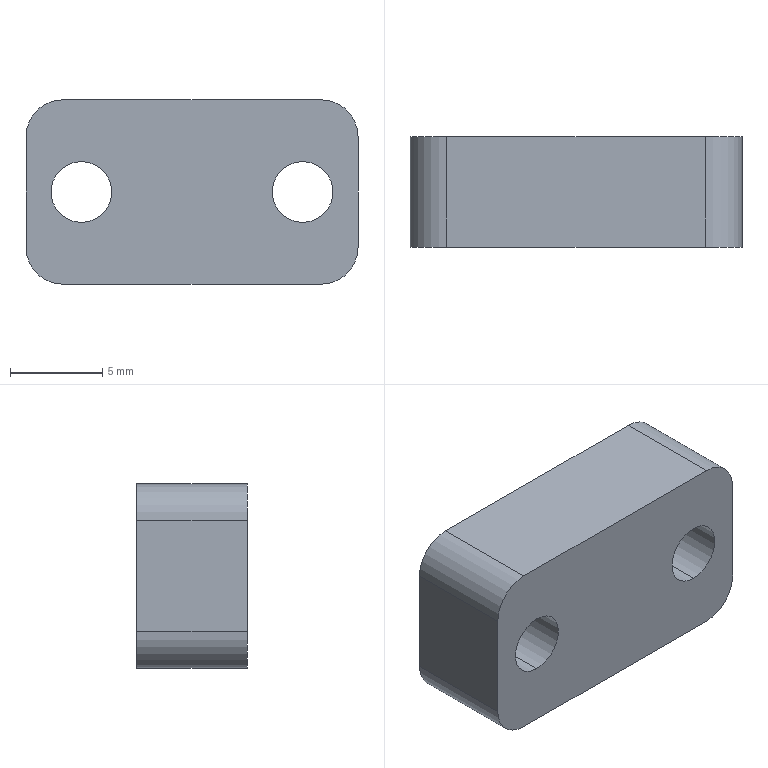Part | SolidWorks | features Extrusion 1, Fillet 1, HoleWzd 1 | 1 solid | 14 faces | box 18 x 6 x 10 mm | volume 956.762 mm3 | cylinder 8 | plane 6 | commonest cylinder face diameters 3.3 x4 4 x4
STEP:
#1=CARTESIAN_POINT('',(-6.,-3.,3.35));
#2=VERTEX_POINT('',#1);
#3=CARTESIAN_POINT('',(-6.,-3.,6.65));
#4=VERTEX_POINT('',#3);
#5=CARTESIAN_POINT('',(-6.,-3.,5.));
#6=DIRECTION('',(0.,1.,0.));
#7=DIRECTION('',(0.,0.,1.));
#8=AXIS2_PLACEMENT_3D('',#5,#6,#7);
#9=CIRCLE('',#8,1.65);
#10=EDGE_CURVE('',#2,#4,#9,.T.);
#11=ORIENTED_EDGE('',*,*,#10,.F.);
#12=CARTESIAN_POINT('',(-6.,3.,3.35));
#13=VERTEX_POINT('',#12);
#14=CARTESIAN_POINT('',(-6.,3.,3.35));
#15=DIRECTION('',(0.,1.,0.));
#16=VECTOR('',#15,1000.);
#17=LINE('',#14,#16);
#18=EDGE_CURVE('',#2,#13,#17,.T.);
#19=ORIENTED_EDGE('',*,*,#18,.T.);
#20=CARTESIAN_POINT('',(-6.,3.,6.65));
#21=VERTEX_POINT('',#20);
#22=CARTESIAN_POINT('',(-6.,3.,5.));
#23=DIRECTION('',(0.,1.,0.));
#24=DIRECTION('',(0.,0.,1.));
#25=AXIS2_PLACEMENT_3D('',#22,#23,#24);
#26=CIRCLE('',#25,1.65);
#27=EDGE_CURVE('',#13,#21,#26,.T.);
#28=ORIENTED_EDGE('',*,*,#27,.T.);
#29=CARTESIAN_POINT('',(-6.,3.,6.65));
#30=DIRECTION('',(0.,1.,0.));
#31=VECTOR('',#30,1000.);
#32=LINE('',#29,#31);
#33=EDGE_CURVE('',#4,#21,#32,.T.);
#34=ORIENTED_EDGE('',*,*,#33,.F.);
#35=EDGE_LOOP('',(#11,#19,#28,#34));
#36=FACE_OUTER_BOUND('',#35,.T.);
#37=CARTESIAN_POINT('',(-6.,3.,5.));
#38=DIRECTION('',(0.,1.,0.));
#39=DIRECTION('',(0.,0.,1.));
#40=AXIS2_PLACEMENT_3D('',#37,#38,#39);
#41=CYLINDRICAL_SURFACE('',#40,1.65);
#42=ADVANCED_FACE('',(#36),#41,.F.);
#43=CARTESIAN_POINT('',(6.,-3.,3.35));
#44=VERTEX_POINT('',#43);
#45=CARTESIAN_POINT('',(6.,-3.,6.65));
#46=VERTEX_POINT('',#45);
#47=CARTESIAN_POINT('',(6.,-3.,5.));
#48=DIRECTION('',(0.,1.,0.));
#49=DIRECTION('',(0.,0.,1.));
#50=AXIS2_PLACEMENT_3D('',#47,#48,#49);
#51=CIRCLE('',#50,1.65);
#52=EDGE_CURVE('',#44,#46,#51,.T.);
#53=ORIENTED_EDGE('',*,*,#52,.F.);
#54=CARTESIAN_POINT('',(6.,3.,3.35));
#55=VERTEX_POINT('',#54);
#56=CARTESIAN_POINT('',(6.,3.,3.35));
#57=DIRECTION('',(0.,1.,0.));
#58=VECTOR('',#57,1000.);
#59=LINE('',#56,#58);
#60=EDGE_CURVE('',#44,#55,#59,.T.);
#61=ORIENTED_EDGE('',*,*,#60,.T.);
#62=CARTESIAN_POINT('',(6.,3.,6.65));
#63=VERTEX_POINT('',#62);
#64=CARTESIAN_POINT('',(6.,3.,5.));
#65=DIRECTION('',(0.,1.,0.));
#66=DIRECTION('',(0.,0.,1.));
#67=AXIS2_PLACEMENT_3D('',#64,#65,#66);
#68=CIRCLE('',#67,1.65);
#69=EDGE_CURVE('',#55,#63,#68,.T.);
#70=ORIENTED_EDGE('',*,*,#69,.T.);
#71=CARTESIAN_POINT('',(6.,3.,6.65));
#72=DIRECTION('',(0.,1.,0.));
#73=VECTOR('',#72,1000.);
#74=LINE('',#71,#73);
#75=EDGE_CURVE('',#46,#63,#74,.T.);
#76=ORIENTED_EDGE('',*,*,#75,.F.);
#77=EDGE_LOOP('',(#53,#61,#70,#76));
#78=FACE_OUTER_BOUND('',#77,.T.);
#79=CARTESIAN_POINT('',(6.,3.,5.));
#80=DIRECTION('',(0.,1.,0.));
#81=DIRECTION('',(0.,0.,1.));
#82=AXIS2_PLACEMENT_3D('',#79,#80,#81);
#83=CYLINDRICAL_SURFACE('',#82,1.65);
#84=ADVANCED_FACE('',(#78),#83,.F.);
#85=CARTESIAN_POINT('',(9.,3.,8.));
#86=VERTEX_POINT('',#85);
#87=CARTESIAN_POINT('',(9.,3.,2.));
#88=VERTEX_POINT('',#87);
#89=CARTESIAN_POINT('',(9.,3.,10.));
#90=DIRECTION('',(0.,0.,-1.));
#91=VECTOR('',#90,1000.);
#92=LINE('',#89,#91);
#93=EDGE_CURVE('',#86,#88,#92,.T.);
#94=ORIENTED_EDGE('',*,*,#93,.F.);
#95=CARTESIAN_POINT('',(9.,-3.,8.));
#96=VERTEX_POINT('',#95);
#97=CARTESIAN_POINT('',(9.,-3.,8.));
#98=DIRECTION('',(0.,-1.,0.));
#99=VECTOR('',#98,1000.);
#100=LINE('',#97,#99);
#101=EDGE_CURVE('',#86,#96,#100,.T.);
#102=ORIENTED_EDGE('',*,*,#101,.T.);
#103=CARTESIAN_POINT('',(9.,-3.,2.));
#104=VERTEX_POINT('',#103);
#105=CARTESIAN_POINT('',(9.,-3.,10.));
#106=DIRECTION('',(0.,0.,-1.));
#107=VECTOR('',#106,1000.);
#108=LINE('',#105,#107);
#109=EDGE_CURVE('',#96,#104,#108,.T.);
#110=ORIENTED_EDGE('',*,*,#109,.T.);
#111=CARTESIAN_POINT('',(9.,3.,2.));
#112=DIRECTION('',(0.,1.,0.));
#113=VECTOR('',#112,1000.);
#114=LINE('',#111,#113);
#115=EDGE_CURVE('',#104,#88,#114,.T.);
#116=ORIENTED_EDGE('',*,*,#115,.T.);
#117=EDGE_LOOP('',(#94,#102,#110,#116));
#118=FACE_OUTER_BOUND('',#117,.T.);
#119=CARTESIAN_POINT('',(9.,-3.,10.));
#120=DIRECTION('',(-1.,0.,0.));
#121=DIRECTION('',(0.,0.,1.));
#122=AXIS2_PLACEMENT_3D('',#119,#120,#121);
#123=PLANE('',#122);
#124=ADVANCED_FACE('',(#118),#123,.F.);
#125=CARTESIAN_POINT('',(-6.,3.,5.));
#126=DIRECTION('',(0.,1.,0.));
#127=DIRECTION('',(0.,0.,1.));
#128=AXIS2_PLACEMENT_3D('',#125,#126,#127);
#129=CIRCLE('',#128,1.65);
#130=EDGE_CURVE('',#21,#13,#129,.T.);
#131=ORIENTED_EDGE('',*,*,#130,.F.);
#132=ORIENTED_EDGE('',*,*,#27,.F.);
#133=EDGE_LOOP('',(#131,#132));
#134=FACE_BOUND('',#133,.T.);
#135=CARTESIAN_POINT('',(6.,3.,5.));
#136=DIRECTION('',(0.,1.,0.));
#137=DIRECTION('',(0.,0.,1.));
#138=AXIS2_PLACEMENT_3D('',#135,#136,#137);
#139=CIRCLE('',#138,1.65);
#140=EDGE_CURVE('',#63,#55,#139,.T.);
#141=ORIENTED_EDGE('',*,*,#140,.F.);
#142=ORIENTED_EDGE('',*,*,#69,.F.);
#143=EDGE_LOOP('',(#141,#142));
#144=FACE_BOUND('',#143,.T.);
#145=CARTESIAN_POINT('',(-9.,3.,8.));
#146=VERTEX_POINT('',#145);
#147=CARTESIAN_POINT('',(-9.,3.,2.));
#148=VERTEX_POINT('',#147);
#149=CARTESIAN_POINT('',(-9.,3.,10.));
#150=DIRECTION('',(0.,0.,-1.));
#151=VECTOR('',#150,1000.);
#152=LINE('',#149,#151);
#153=EDGE_CURVE('',#146,#148,#152,.T.);
#154=ORIENTED_EDGE('',*,*,#153,.F.);
#155=CARTESIAN_POINT('',(-7.,3.,10.));
#156=VERTEX_POINT('',#155);
#157=CARTESIAN_POINT('',(-7.,3.,8.));
#158=DIRECTION('',(0.,1.,0.));
#159=DIRECTION('',(0.,0.,-1.));
#160=AXIS2_PLACEMENT_3D('',#157,#158,#159);
#161=CIRCLE('',#160,2.);
#162=EDGE_CURVE('',#146,#156,#161,.T.);
#163=ORIENTED_EDGE('',*,*,#162,.T.);
#164=CARTESIAN_POINT('',(7.,3.,10.));
#165=VERTEX_POINT('',#164);
#166=CARTESIAN_POINT('',(-9.,3.,10.));
#167=DIRECTION('',(-1.,0.,0.));
#168=VECTOR('',#167,1000.);
#169=LINE('',#166,#168);
#170=EDGE_CURVE('',#165,#156,#169,.T.);
#171=ORIENTED_EDGE('',*,*,#170,.F.);
#172=CARTESIAN_POINT('',(7.,3.,8.));
#173=DIRECTION('',(0.,1.,0.));
#174=DIRECTION('',(0.,0.,-1.));
#175=AXIS2_PLACEMENT_3D('',#172,#173,#174);
#176=CIRCLE('',#175,2.);
#177=EDGE_CURVE('',#165,#86,#176,.T.);
#178=ORIENTED_EDGE('',*,*,#177,.T.);
#179=ORIENTED_EDGE('',*,*,#93,.T.);
#180=CARTESIAN_POINT('',(7.,3.,0.));
#181=VERTEX_POINT('',#180);
#182=CARTESIAN_POINT('',(7.,3.,2.));
#183=DIRECTION('',(0.,1.,0.));
#184=DIRECTION('',(0.,0.,-1.));
#185=AXIS2_PLACEMENT_3D('',#182,#183,#184);
#186=CIRCLE('',#185,2.);
#187=EDGE_CURVE('',#88,#181,#186,.T.);
#188=ORIENTED_EDGE('',*,*,#187,.T.);
#189=CARTESIAN_POINT('',(-7.,3.,0.));
#190=VERTEX_POINT('',#189);
#191=CARTESIAN_POINT('',(-9.,3.,0.));
#192=DIRECTION('',(-1.,0.,0.));
#193=VECTOR('',#192,1000.);
#194=LINE('',#191,#193);
#195=EDGE_CURVE('',#181,#190,#194,.T.);
#196=ORIENTED_EDGE('',*,*,#195,.T.);
#197=CARTESIAN_POINT('',(-7.,3.,2.));
#198=DIRECTION('',(0.,1.,0.));
#199=DIRECTION('',(0.,0.,-1.));
#200=AXIS2_PLACEMENT_3D('',#197,#198,#199);
#201=CIRCLE('',#200,2.);
#202=EDGE_CURVE('',#190,#148,#201,.T.);
#203=ORIENTED_EDGE('',*,*,#202,.T.);
#204=EDGE_LOOP('',(#154,#163,#171,#178,#179,#188,#196,#203));
#205=FACE_OUTER_BOUND('',#204,.T.);
#206=CARTESIAN_POINT('',(-9.,3.,10.));
#207=DIRECTION('',(0.,-1.,0.));
#208=DIRECTION('',(0.,0.,-1.));
#209=AXIS2_PLACEMENT_3D('',#206,#207,#208);
#210=PLANE('',#209);
#211=ADVANCED_FACE('',(#134,#144,#205),#210,.F.);
#212=CARTESIAN_POINT('',(-9.,-3.,8.));
#213=VERTEX_POINT('',#212);
#214=CARTESIAN_POINT('',(-9.,-3.,2.));
#215=VERTEX_POINT('',#214);
#216=CARTESIAN_POINT('',(-9.,-3.,10.));
#217=DIRECTION('',(0.,0.,-1.));
#218=VECTOR('',#217,1000.);
#219=LINE('',#216,#218);
#220=EDGE_CURVE('',#213,#215,#219,.T.);
#221=ORIENTED_EDGE('',*,*,#220,.F.);
#222=CARTESIAN_POINT('',(-9.,-3.,8.));
#223=DIRECTION('',(0.,1.,0.));
#224=VECTOR('',#223,1000.);
#225=LINE('',#222,#224);
#226=EDGE_CURVE('',#213,#146,#225,.T.);
#227=ORIENTED_EDGE('',*,*,#226,.T.);
#228=ORIENTED_EDGE('',*,*,#153,.T.);
#229=CARTESIAN_POINT('',(-9.,-3.,2.));
#230=DIRECTION('',(0.,-1.,0.));
#231=VECTOR('',#230,1000.);
#232=LINE('',#229,#231);
#233=EDGE_CURVE('',#148,#215,#232,.T.);
#234=ORIENTED_EDGE('',*,*,#233,.T.);
#235=EDGE_LOOP('',(#221,#227,#228,#234));
#236=FACE_OUTER_BOUND('',#235,.T.);
#237=CARTESIAN_POINT('',(-9.,-3.,10.));
#238=DIRECTION('',(1.,0.,0.));
#239=DIRECTION('',(0.,0.,-1.));
#240=AXIS2_PLACEMENT_3D('',#237,#238,#239);
#241=PLANE('',#240);
#242=ADVANCED_FACE('',(#236),#241,.F.);
#243=CARTESIAN_POINT('',(-6.,-3.,5.));
#244=DIRECTION('',(0.,1.,0.));
#245=DIRECTION('',(0.,0.,1.));
#246=AXIS2_PLACEMENT_3D('',#243,#244,#245);
#247=CIRCLE('',#246,1.65);
#248=EDGE_CURVE('',#4,#2,#247,.T.);
#249=ORIENTED_EDGE('',*,*,#248,.T.);
#250=ORIENTED_EDGE('',*,*,#10,.T.);
#251=EDGE_LOOP('',(#249,#250));
#252=FACE_BOUND('',#251,.T.);
#253=CARTESIAN_POINT('',(6.,-3.,5.));
#254=DIRECTION('',(0.,1.,0.));
#255=DIRECTION('',(0.,0.,1.));
#256=AXIS2_PLACEMENT_3D('',#253,#254,#255);
#257=CIRCLE('',#256,1.65);
#258=EDGE_CURVE('',#46,#44,#257,.T.);
#259=ORIENTED_EDGE('',*,*,#258,.T.);
#260=ORIENTED_EDGE('',*,*,#52,.T.);
#261=EDGE_LOOP('',(#259,#260));
#262=FACE_BOUND('',#261,.T.);
#263=CARTESIAN_POINT('',(-7.,-3.,10.));
#264=VERTEX_POINT('',#263);
#265=CARTESIAN_POINT('',(7.,-3.,10.));
#266=VERTEX_POINT('',#265);
#267=CARTESIAN_POINT('',(-9.,-3.,10.));
#268=DIRECTION('',(1.,0.,0.));
#269=VECTOR('',#268,1000.);
#270=LINE('',#267,#269);
#271=EDGE_CURVE('',#264,#266,#270,.T.);
#272=ORIENTED_EDGE('',*,*,#271,.F.);
#273=CARTESIAN_POINT('',(-7.,-3.,8.));
#274=DIRECTION('',(0.,-1.,0.));
#275=DIRECTION('',(0.,0.,1.));
#276=AXIS2_PLACEMENT_3D('',#273,#274,#275);
#277=CIRCLE('',#276,2.);
#278=EDGE_CURVE('',#264,#213,#277,.T.);
#279=ORIENTED_EDGE('',*,*,#278,.T.);
#280=ORIENTED_EDGE('',*,*,#220,.T.);
#281=CARTESIAN_POINT('',(-7.,-3.,0.));
#282=VERTEX_POINT('',#281);
#283=CARTESIAN_POINT('',(-7.,-3.,2.));
#284=DIRECTION('',(0.,-1.,0.));
#285=DIRECTION('',(0.,0.,1.));
#286=AXIS2_PLACEMENT_3D('',#283,#284,#285);
#287=CIRCLE('',#286,2.);
#288=EDGE_CURVE('',#215,#282,#287,.T.);
#289=ORIENTED_EDGE('',*,*,#288,.T.);
#290=CARTESIAN_POINT('',(7.,-3.,0.));
#291=VERTEX_POINT('',#290);
#292=CARTESIAN_POINT('',(-9.,-3.,0.));
#293=DIRECTION('',(1.,0.,0.));
#294=VECTOR('',#293,1000.);
#295=LINE('',#292,#294);
#296=EDGE_CURVE('',#282,#291,#295,.T.);
#297=ORIENTED_EDGE('',*,*,#296,.T.);
#298=CARTESIAN_POINT('',(7.,-3.,2.));
#299=DIRECTION('',(0.,-1.,0.));
#300=DIRECTION('',(0.,0.,1.));
#301=AXIS2_PLACEMENT_3D('',#298,#299,#300);
#302=CIRCLE('',#301,2.);
#303=EDGE_CURVE('',#291,#104,#302,.T.);
#304=ORIENTED_EDGE('',*,*,#303,.T.);
#305=ORIENTED_EDGE('',*,*,#109,.F.);
#306=CARTESIAN_POINT('',(7.,-3.,8.));
#307=DIRECTION('',(0.,-1.,0.));
#308=DIRECTION('',(0.,0.,1.));
#309=AXIS2_PLACEMENT_3D('',#306,#307,#308);
#310=CIRCLE('',#309,2.);
#311=EDGE_CURVE('',#96,#266,#310,.T.);
#312=ORIENTED_EDGE('',*,*,#311,.T.);
#313=EDGE_LOOP('',(#272,#279,#280,#289,#297,#304,#305,#312));
#314=FACE_OUTER_BOUND('',#313,.T.);
#315=CARTESIAN_POINT('',(-9.,-3.,10.));
#316=DIRECTION('',(0.,1.,0.));
#317=DIRECTION('',(0.,0.,1.));
#318=AXIS2_PLACEMENT_3D('',#315,#316,#317);
#319=PLANE('',#318);
#320=ADVANCED_FACE('',(#252,#262,#314),#319,.F.);
#321=ORIENTED_EDGE('',*,*,#170,.T.);
#322=CARTESIAN_POINT('',(-7.,0.,10.));
#323=DIRECTION('',(0.,-1.,0.));
#324=VECTOR('',#323,1000.);
#325=LINE('',#322,#324);
#326=EDGE_CURVE('',#156,#264,#325,.T.);
#327=ORIENTED_EDGE('',*,*,#326,.T.);
#328=ORIENTED_EDGE('',*,*,#271,.T.);
#329=CARTESIAN_POINT('',(7.,0.,10.));
#330=DIRECTION('',(0.,1.,0.));
#331=VECTOR('',#330,1000.);
#332=LINE('',#329,#331);
#333=EDGE_CURVE('',#266,#165,#332,.T.);
#334=ORIENTED_EDGE('',*,*,#333,.T.);
#335=EDGE_LOOP('',(#321,#327,#328,#334));
#336=FACE_OUTER_BOUND('',#335,.T.);
#337=CARTESIAN_POINT('',(0.,0.,10.));
#338=DIRECTION('',(0.,0.,-1.));
#339=DIRECTION('',(-1.,0.,0.));
#340=AXIS2_PLACEMENT_3D('',#337,#338,#339);
#341=PLANE('',#340);
#342=ADVANCED_FACE('',(#336),#341,.F.);
#343=ORIENTED_EDGE('',*,*,#195,.F.);
#344=CARTESIAN_POINT('',(7.,-3.,0.));
#345=DIRECTION('',(0.,-1.,0.));
#346=VECTOR('',#345,1000.);
#347=LINE('',#344,#346);
#348=EDGE_CURVE('',#181,#291,#347,.T.);
#349=ORIENTED_EDGE('',*,*,#348,.T.);
#350=ORIENTED_EDGE('',*,*,#296,.F.);
#351=CARTESIAN_POINT('',(-7.,3.,0.));
#352=DIRECTION('',(0.,1.,0.));
#353=VECTOR('',#352,1000.);
#354=LINE('',#351,#353);
#355=EDGE_CURVE('',#282,#190,#354,.T.);
#356=ORIENTED_EDGE('',*,*,#355,.T.);
#357=EDGE_LOOP('',(#343,#349,#350,#356));
#358=FACE_OUTER_BOUND('',#357,.T.);
#359=CARTESIAN_POINT('',(0.,0.,0.));
#360=DIRECTION('',(0.,0.,-1.));
#361=DIRECTION('',(-1.,0.,0.));
#362=AXIS2_PLACEMENT_3D('',#359,#360,#361);
#363=PLANE('',#362);
#364=ADVANCED_FACE('',(#358),#363,.T.);
#365=ORIENTED_EDGE('',*,*,#60,.F.);
#366=ORIENTED_EDGE('',*,*,#258,.F.);
#367=ORIENTED_EDGE('',*,*,#75,.T.);
#368=ORIENTED_EDGE('',*,*,#140,.T.);
#369=EDGE_LOOP('',(#365,#366,#367,#368));
#370=FACE_OUTER_BOUND('',#369,.T.);
#371=CARTESIAN_POINT('',(6.,3.,5.));
#372=DIRECTION('',(0.,1.,0.));
#373=DIRECTION('',(0.,0.,1.));
#374=AXIS2_PLACEMENT_3D('',#371,#372,#373);
#375=CYLINDRICAL_SURFACE('',#374,1.65);
#376=ADVANCED_FACE('',(#370),#375,.F.);
#377=ORIENTED_EDGE('',*,*,#18,.F.);
#378=ORIENTED_EDGE('',*,*,#248,.F.);
#379=ORIENTED_EDGE('',*,*,#33,.T.);
#380=ORIENTED_EDGE('',*,*,#130,.T.);
#381=EDGE_LOOP('',(#377,#378,#379,#380));
#382=FACE_OUTER_BOUND('',#381,.T.);
#383=CARTESIAN_POINT('',(-6.,3.,5.));
#384=DIRECTION('',(0.,1.,0.));
#385=DIRECTION('',(0.,0.,1.));
#386=AXIS2_PLACEMENT_3D('',#383,#384,#385);
#387=CYLINDRICAL_SURFACE('',#386,1.65);
#388=ADVANCED_FACE('',(#382),#387,.F.);
#389=ORIENTED_EDGE('',*,*,#162,.F.);
#390=ORIENTED_EDGE('',*,*,#226,.F.);
#391=ORIENTED_EDGE('',*,*,#278,.F.);
#392=ORIENTED_EDGE('',*,*,#326,.F.);
#393=EDGE_LOOP('',(#389,#390,#391,#392));
#394=FACE_OUTER_BOUND('',#393,.T.);
#395=CARTESIAN_POINT('',(-7.,0.,8.));
#396=DIRECTION('',(0.,-1.,0.));
#397=DIRECTION('',(0.,0.,-1.));
#398=AXIS2_PLACEMENT_3D('',#395,#396,#397);
#399=CYLINDRICAL_SURFACE('',#398,2.);
#400=ADVANCED_FACE('',(#394),#399,.T.);
#401=ORIENTED_EDGE('',*,*,#311,.F.);
#402=ORIENTED_EDGE('',*,*,#101,.F.);
#403=ORIENTED_EDGE('',*,*,#177,.F.);
#404=ORIENTED_EDGE('',*,*,#333,.F.);
#405=EDGE_LOOP('',(#401,#402,#403,#404));
#406=FACE_OUTER_BOUND('',#405,.T.);
#407=CARTESIAN_POINT('',(7.,0.,8.));
#408=DIRECTION('',(0.,1.,0.));
#409=DIRECTION('',(0.,0.,1.));
#410=AXIS2_PLACEMENT_3D('',#407,#408,#409);
#411=CYLINDRICAL_SURFACE('',#410,2.);
#412=ADVANCED_FACE('',(#406),#411,.T.);
#413=ORIENTED_EDGE('',*,*,#303,.F.);
#414=ORIENTED_EDGE('',*,*,#348,.F.);
#415=ORIENTED_EDGE('',*,*,#187,.F.);
#416=ORIENTED_EDGE('',*,*,#115,.F.);
#417=EDGE_LOOP('',(#413,#414,#415,#416));
#418=FACE_OUTER_BOUND('',#417,.T.);
#419=CARTESIAN_POINT('',(7.,-3.,2.));
#420=DIRECTION('',(0.,-1.,0.));
#421=DIRECTION('',(0.,0.,-1.));
#422=AXIS2_PLACEMENT_3D('',#419,#420,#421);
#423=CYLINDRICAL_SURFACE('',#422,2.);
#424=ADVANCED_FACE('',(#418),#423,.T.);
#425=ORIENTED_EDGE('',*,*,#202,.F.);
#426=ORIENTED_EDGE('',*,*,#355,.F.);
#427=ORIENTED_EDGE('',*,*,#288,.F.);
#428=ORIENTED_EDGE('',*,*,#233,.F.);
#429=EDGE_LOOP('',(#425,#426,#427,#428));
#430=FACE_OUTER_BOUND('',#429,.T.);
#431=CARTESIAN_POINT('',(-7.,-3.,2.));
#432=DIRECTION('',(0.,1.,0.));
#433=DIRECTION('',(0.,0.,1.));
#434=AXIS2_PLACEMENT_3D('',#431,#432,#433);
#435=CYLINDRICAL_SURFACE('',#434,2.);
#436=ADVANCED_FACE('',(#430),#435,.T.);
#437=CLOSED_SHELL('',(#42,#84,#124,#211,#242,#320,#342,#364,#376,#388,#400,#412,#424,#436));
#438=MANIFOLD_SOLID_BREP('',#437);
#439=CARTESIAN_POINT('',(0.,0.,0.));
#440=DIRECTION('',(0.,0.,1.));
#441=DIRECTION('',(1.,0.,0.));
#442=AXIS2_PLACEMENT_3D('',#439,#440,#441);
#443=(LENGTH_UNIT()NAMED_UNIT(*)SI_UNIT(.MILLI.,.METRE.));
#444=UNCERTAINTY_MEASURE_WITH_UNIT(LENGTH_MEASURE(0.00001),#443,'','');
#445=(NAMED_UNIT(*)PLANE_ANGLE_UNIT()SI_UNIT($,.RADIAN.));
#446=(NAMED_UNIT(*)SI_UNIT($,.STERADIAN.)SOLID_ANGLE_UNIT());
#447=(GEOMETRIC_REPRESENTATION_CONTEXT(3)GLOBAL_UNCERTAINTY_ASSIGNED_CONTEXT((#444))GLOBAL_UNIT_ASSIGNED_CONTEXT((#443,#445,#446))REPRESENTATION_CONTEXT('',''));
#448=ADVANCED_BREP_SHAPE_REPRESENTATION('',(#438,#442),#447);